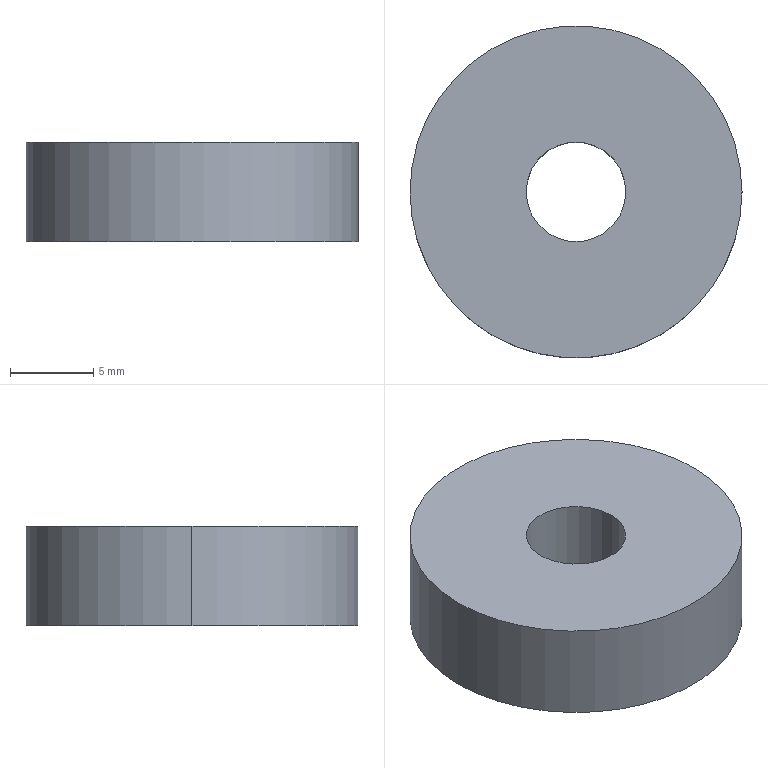Part | SolidWorks | features Extrusion 1 | 1 solid | 6 faces | box 20 x 20 x 6 mm | volume 1715 mm3 | cylinder 4 | plane 2 | commonest cylinder face diameters 6 x2 20 x2
STEP:
#1=CARTESIAN_POINT('',(-3.,0.,6.));
#2=VERTEX_POINT('',#1);
#3=CARTESIAN_POINT('',(3.,0.,6.));
#4=VERTEX_POINT('',#3);
#5=CARTESIAN_POINT('',(0.,0.,6.));
#6=DIRECTION('',(0.,0.,1.));
#7=DIRECTION('',(1.,0.,0.));
#8=AXIS2_PLACEMENT_3D('',#5,#6,#7);
#9=CIRCLE('',#8,3.);
#10=EDGE_CURVE('',#2,#4,#9,.T.);
#11=ORIENTED_EDGE('',*,*,#10,.T.);
#12=CARTESIAN_POINT('',(3.,0.,0.));
#13=VERTEX_POINT('',#12);
#14=CARTESIAN_POINT('',(3.,0.,6.));
#15=DIRECTION('',(0.,0.,-1.));
#16=VECTOR('',#15,1000.);
#17=LINE('',#14,#16);
#18=EDGE_CURVE('',#4,#13,#17,.T.);
#19=ORIENTED_EDGE('',*,*,#18,.T.);
#20=CARTESIAN_POINT('',(-3.,0.,0.));
#21=VERTEX_POINT('',#20);
#22=CARTESIAN_POINT('',(0.,0.,0.));
#23=DIRECTION('',(0.,0.,1.));
#24=DIRECTION('',(1.,0.,0.));
#25=AXIS2_PLACEMENT_3D('',#22,#23,#24);
#26=CIRCLE('',#25,3.);
#27=EDGE_CURVE('',#21,#13,#26,.T.);
#28=ORIENTED_EDGE('',*,*,#27,.F.);
#29=CARTESIAN_POINT('',(-3.,0.,6.));
#30=DIRECTION('',(0.,0.,-1.));
#31=VECTOR('',#30,1000.);
#32=LINE('',#29,#31);
#33=EDGE_CURVE('',#2,#21,#32,.T.);
#34=ORIENTED_EDGE('',*,*,#33,.F.);
#35=EDGE_LOOP('',(#11,#19,#28,#34));
#36=FACE_OUTER_BOUND('',#35,.T.);
#37=CARTESIAN_POINT('',(0.,0.,6.));
#38=DIRECTION('',(0.,0.,-1.));
#39=DIRECTION('',(-1.,0.,0.));
#40=AXIS2_PLACEMENT_3D('',#37,#38,#39);
#41=CYLINDRICAL_SURFACE('',#40,3.);
#42=ADVANCED_FACE('',(#36),#41,.F.);
#43=CARTESIAN_POINT('',(10.,0.,6.));
#44=VERTEX_POINT('',#43);
#45=CARTESIAN_POINT('',(-10.,0.,6.));
#46=VERTEX_POINT('',#45);
#47=CARTESIAN_POINT('',(0.,0.,6.));
#48=DIRECTION('',(0.,0.,1.));
#49=DIRECTION('',(1.,0.,0.));
#50=AXIS2_PLACEMENT_3D('',#47,#48,#49);
#51=CIRCLE('',#50,10.);
#52=EDGE_CURVE('',#44,#46,#51,.T.);
#53=ORIENTED_EDGE('',*,*,#52,.F.);
#54=CARTESIAN_POINT('',(10.,0.,0.));
#55=VERTEX_POINT('',#54);
#56=CARTESIAN_POINT('',(10.,0.,6.));
#57=DIRECTION('',(0.,0.,-1.));
#58=VECTOR('',#57,1000.);
#59=LINE('',#56,#58);
#60=EDGE_CURVE('',#44,#55,#59,.T.);
#61=ORIENTED_EDGE('',*,*,#60,.T.);
#62=CARTESIAN_POINT('',(-10.,0.,0.));
#63=VERTEX_POINT('',#62);
#64=CARTESIAN_POINT('',(0.,0.,0.));
#65=DIRECTION('',(0.,0.,1.));
#66=DIRECTION('',(1.,0.,0.));
#67=AXIS2_PLACEMENT_3D('',#64,#65,#66);
#68=CIRCLE('',#67,10.);
#69=EDGE_CURVE('',#55,#63,#68,.T.);
#70=ORIENTED_EDGE('',*,*,#69,.T.);
#71=CARTESIAN_POINT('',(-10.,0.,6.));
#72=DIRECTION('',(0.,0.,-1.));
#73=VECTOR('',#72,1000.);
#74=LINE('',#71,#73);
#75=EDGE_CURVE('',#46,#63,#74,.T.);
#76=ORIENTED_EDGE('',*,*,#75,.F.);
#77=EDGE_LOOP('',(#53,#61,#70,#76));
#78=FACE_OUTER_BOUND('',#77,.T.);
#79=CARTESIAN_POINT('',(0.,0.,6.));
#80=DIRECTION('',(0.,0.,-1.));
#81=DIRECTION('',(-1.,0.,0.));
#82=AXIS2_PLACEMENT_3D('',#79,#80,#81);
#83=CYLINDRICAL_SURFACE('',#82,10.);
#84=ADVANCED_FACE('',(#78),#83,.T.);
#85=CARTESIAN_POINT('',(0.,0.,6.));
#86=DIRECTION('',(0.,0.,1.));
#87=DIRECTION('',(1.,0.,0.));
#88=AXIS2_PLACEMENT_3D('',#85,#86,#87);
#89=CIRCLE('',#88,10.);
#90=EDGE_CURVE('',#46,#44,#89,.T.);
#91=ORIENTED_EDGE('',*,*,#90,.T.);
#92=ORIENTED_EDGE('',*,*,#52,.T.);
#93=EDGE_LOOP('',(#91,#92));
#94=FACE_OUTER_BOUND('',#93,.T.);
#95=ORIENTED_EDGE('',*,*,#10,.F.);
#96=CARTESIAN_POINT('',(0.,0.,6.));
#97=DIRECTION('',(0.,0.,1.));
#98=DIRECTION('',(1.,0.,0.));
#99=AXIS2_PLACEMENT_3D('',#96,#97,#98);
#100=CIRCLE('',#99,3.);
#101=EDGE_CURVE('',#4,#2,#100,.T.);
#102=ORIENTED_EDGE('',*,*,#101,.F.);
#103=EDGE_LOOP('',(#95,#102));
#104=FACE_BOUND('',#103,.T.);
#105=CARTESIAN_POINT('',(0.,0.,6.));
#106=DIRECTION('',(0.,0.,1.));
#107=DIRECTION('',(1.,0.,0.));
#108=AXIS2_PLACEMENT_3D('',#105,#106,#107);
#109=PLANE('',#108);
#110=ADVANCED_FACE('',(#94,#104),#109,.T.);
#111=CARTESIAN_POINT('',(0.,0.,0.));
#112=DIRECTION('',(0.,0.,1.));
#113=DIRECTION('',(1.,0.,0.));
#114=AXIS2_PLACEMENT_3D('',#111,#112,#113);
#115=CIRCLE('',#114,10.);
#116=EDGE_CURVE('',#63,#55,#115,.T.);
#117=ORIENTED_EDGE('',*,*,#116,.F.);
#118=ORIENTED_EDGE('',*,*,#69,.F.);
#119=EDGE_LOOP('',(#117,#118));
#120=FACE_OUTER_BOUND('',#119,.T.);
#121=ORIENTED_EDGE('',*,*,#27,.T.);
#122=CARTESIAN_POINT('',(0.,0.,0.));
#123=DIRECTION('',(0.,0.,1.));
#124=DIRECTION('',(1.,0.,0.));
#125=AXIS2_PLACEMENT_3D('',#122,#123,#124);
#126=CIRCLE('',#125,3.);
#127=EDGE_CURVE('',#13,#21,#126,.T.);
#128=ORIENTED_EDGE('',*,*,#127,.T.);
#129=EDGE_LOOP('',(#121,#128));
#130=FACE_BOUND('',#129,.T.);
#131=CARTESIAN_POINT('',(0.,0.,0.));
#132=DIRECTION('',(0.,0.,1.));
#133=DIRECTION('',(1.,0.,0.));
#134=AXIS2_PLACEMENT_3D('',#131,#132,#133);
#135=PLANE('',#134);
#136=ADVANCED_FACE('',(#120,#130),#135,.F.);
#137=ORIENTED_EDGE('',*,*,#60,.F.);
#138=ORIENTED_EDGE('',*,*,#90,.F.);
#139=ORIENTED_EDGE('',*,*,#75,.T.);
#140=ORIENTED_EDGE('',*,*,#116,.T.);
#141=EDGE_LOOP('',(#137,#138,#139,#140));
#142=FACE_OUTER_BOUND('',#141,.T.);
#143=CARTESIAN_POINT('',(0.,0.,6.));
#144=DIRECTION('',(0.,0.,-1.));
#145=DIRECTION('',(-1.,0.,0.));
#146=AXIS2_PLACEMENT_3D('',#143,#144,#145);
#147=CYLINDRICAL_SURFACE('',#146,10.);
#148=ADVANCED_FACE('',(#142),#147,.T.);
#149=ORIENTED_EDGE('',*,*,#18,.F.);
#150=ORIENTED_EDGE('',*,*,#101,.T.);
#151=ORIENTED_EDGE('',*,*,#33,.T.);
#152=ORIENTED_EDGE('',*,*,#127,.F.);
#153=EDGE_LOOP('',(#149,#150,#151,#152));
#154=FACE_OUTER_BOUND('',#153,.T.);
#155=CARTESIAN_POINT('',(0.,0.,6.));
#156=DIRECTION('',(0.,0.,-1.));
#157=DIRECTION('',(-1.,0.,0.));
#158=AXIS2_PLACEMENT_3D('',#155,#156,#157);
#159=CYLINDRICAL_SURFACE('',#158,3.);
#160=ADVANCED_FACE('',(#154),#159,.F.);
#161=CLOSED_SHELL('',(#42,#84,#110,#136,#148,#160));
#162=MANIFOLD_SOLID_BREP('',#161);
#163=CARTESIAN_POINT('',(0.,0.,0.));
#164=DIRECTION('',(0.,0.,1.));
#165=DIRECTION('',(1.,0.,0.));
#166=AXIS2_PLACEMENT_3D('',#163,#164,#165);
#167=(LENGTH_UNIT()NAMED_UNIT(*)SI_UNIT(.MILLI.,.METRE.));
#168=UNCERTAINTY_MEASURE_WITH_UNIT(LENGTH_MEASURE(0.00001),#167,'','');
#169=(NAMED_UNIT(*)PLANE_ANGLE_UNIT()SI_UNIT($,.RADIAN.));
#170=(NAMED_UNIT(*)SI_UNIT($,.STERADIAN.)SOLID_ANGLE_UNIT());
#171=(GEOMETRIC_REPRESENTATION_CONTEXT(3)GLOBAL_UNCERTAINTY_ASSIGNED_CONTEXT((#168))GLOBAL_UNIT_ASSIGNED_CONTEXT((#167,#169,#170))REPRESENTATION_CONTEXT('',''));
#172=ADVANCED_BREP_SHAPE_REPRESENTATION('',(#162,#166),#171);